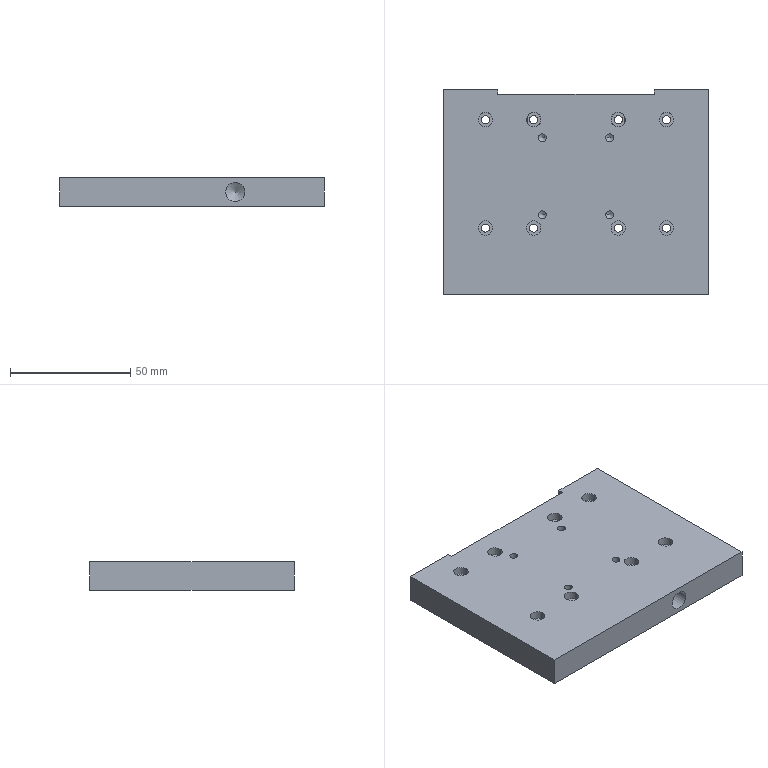Part | NX | features 00 2 | 1 solid | 76 faces | box 110 x 85 x 12 mm | volume 106361 mm3 | cylinder 45 | plane 18 | cone 13 | commonest cylinder face diameters 3.4 x16 6 x16 3.3 x8 6.8 x4 8 x1